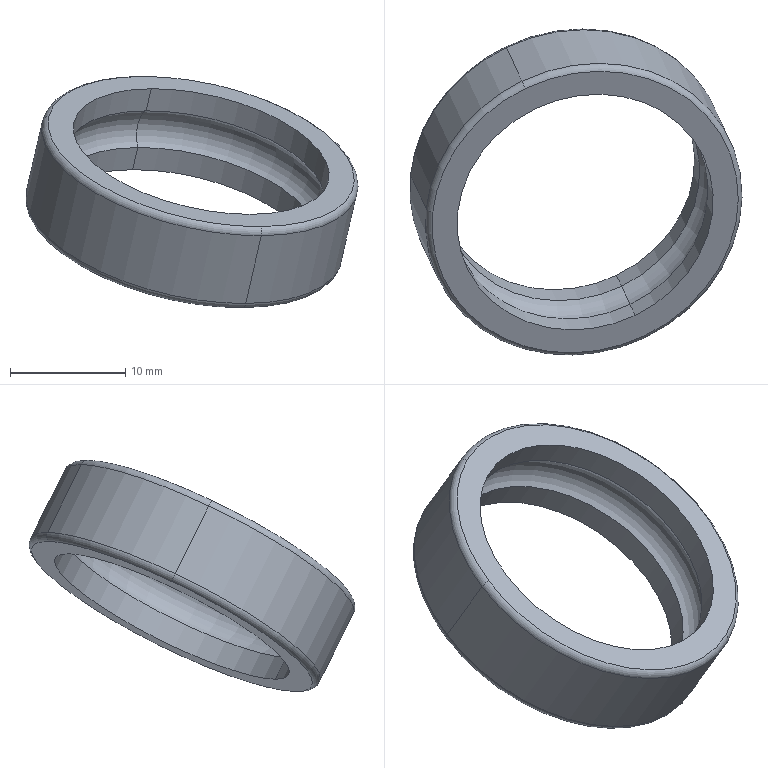Part | SolidWorks | features BaseBody 1 | 1 solid | 20 faces | box 28.804 x 28.259 x 20.047 mm | volume 1513 mm3 | cylinder 9 | torus 9 | plane 2 | commonest cylinder face diameters 22.668 x6 28 x3
STEP:
#1=CARTESIAN_POINT('',(1918.977,-164.664,836.807));
#2=VERTEX_POINT('',#1);
#3=CARTESIAN_POINT('',(1934.349,-173.615,828.827));
#4=VERTEX_POINT('',#3);
#5=CARTESIAN_POINT('',(1930.024,-164.664,834.27));
#6=DIRECTION('',(0.2015,-0.436,0.8771));
#7=DIRECTION('',(-0.3816,0.7898,0.4803));
#8=AXIS2_PLACEMENT_3D('',#5,#6,#7);
#9=CIRCLE('',#8,11.334);
#10=EDGE_CURVE('',#2,#4,#9,.T.);
#11=ORIENTED_EDGE('',*,*,#10,.F.);
#12=CARTESIAN_POINT('',(1919.418,-165.618,838.726));
#13=VERTEX_POINT('',#12);
#14=CARTESIAN_POINT('',(1918.965,-164.637,836.755));
#15=DIRECTION('',(0.2015,-0.436,0.8771));
#16=VECTOR('',#15,1000.);
#17=LINE('',#14,#16);
#18=EDGE_CURVE('',#2,#13,#17,.T.);
#19=ORIENTED_EDGE('',*,*,#18,.T.);
#20=CARTESIAN_POINT('',(1934.79,-174.569,830.746));
#21=VERTEX_POINT('',#20);
#22=CARTESIAN_POINT('',(1930.465,-165.618,836.189));
#23=DIRECTION('',(-0.2015,0.436,-0.8771));
#24=DIRECTION('',(0.3816,-0.7898,-0.4803));
#25=AXIS2_PLACEMENT_3D('',#22,#23,#24);
#26=CIRCLE('',#25,11.334);
#27=EDGE_CURVE('',#21,#13,#26,.T.);
#28=ORIENTED_EDGE('',*,*,#27,.F.);
#29=CARTESIAN_POINT('',(1934.349,-173.615,828.827));
#30=DIRECTION('',(-0.2015,0.436,-0.8771));
#31=VECTOR('',#30,1000.);
#32=LINE('',#29,#31);
#33=EDGE_CURVE('',#21,#4,#32,.T.);
#34=ORIENTED_EDGE('',*,*,#33,.T.);
#35=EDGE_LOOP('',(#11,#19,#28,#34));
#36=FACE_OUTER_BOUND('',#35,.T.);
#37=CARTESIAN_POINT('',(1930.012,-164.637,834.217));
#38=DIRECTION('',(0.2015,-0.436,0.8771));
#39=DIRECTION('',(-0.9746,0.,0.2239));
#40=AXIS2_PLACEMENT_3D('',#37,#38,#39);
#41=CYLINDRICAL_SURFACE('',#40,11.334);
#42=ADVANCED_FACE('',(#36),#41,.F.);
#43=CARTESIAN_POINT('',(1916.818,-164.664,837.303));
#44=VERTEX_POINT('',#43);
#45=CARTESIAN_POINT('',(1924.853,-153.962,840.777));
#46=VERTEX_POINT('',#45);
#47=CARTESIAN_POINT('',(1930.024,-164.664,834.27));
#48=DIRECTION('',(-0.2015,0.436,-0.8771));
#49=DIRECTION('',(0.3816,-0.7898,-0.4803));
#50=AXIS2_PLACEMENT_3D('',#47,#48,#49);
#51=CIRCLE('',#50,13.55);
#52=EDGE_CURVE('',#44,#46,#51,.T.);
#53=ORIENTED_EDGE('',*,*,#52,.F.);
#54=CARTESIAN_POINT('',(1916.51,-164.947,837.974));
#55=VERTEX_POINT('',#54);
#56=CARTESIAN_POINT('',(1917.187,-164.947,837.819));
#57=DIRECTION('',(0.09761,0.8999,0.425));
#58=DIRECTION('',(0.,-0.427,0.9043));
#59=AXIS2_PLACEMENT_3D('',#56,#57,#58);
#60=CIRCLE('',#59,0.6944);
#61=EDGE_CURVE('',#44,#55,#60,.T.);
#62=ORIENTED_EDGE('',*,*,#61,.T.);
#63=CARTESIAN_POINT('',(1924.812,-153.89,841.564));
#64=VERTEX_POINT('',#63);
#65=CARTESIAN_POINT('',(1930.155,-164.947,834.84));
#66=DIRECTION('',(-0.2015,0.436,-0.8771));
#67=DIRECTION('',(0.3816,-0.7898,-0.4803));
#68=AXIS2_PLACEMENT_3D('',#65,#66,#67);
#69=CIRCLE('',#68,14.);
#70=EDGE_CURVE('',#55,#64,#69,.T.);
#71=ORIENTED_EDGE('',*,*,#70,.T.);
#72=CARTESIAN_POINT('',(1925.077,-154.439,841.23));
#73=DIRECTION('',(0.9021,0.4315,0.007269));
#74=DIRECTION('',(-0.3816,0.7898,0.4803));
#75=AXIS2_PLACEMENT_3D('',#72,#73,#74);
#76=CIRCLE('',#75,0.6944);
#77=EDGE_CURVE('',#46,#64,#76,.T.);
#78=ORIENTED_EDGE('',*,*,#77,.F.);
#79=EDGE_LOOP('',(#53,#62,#71,#78));
#80=FACE_OUTER_BOUND('',#79,.T.);
#81=CARTESIAN_POINT('',(1930.155,-164.947,834.84));
#82=DIRECTION('',(0.2015,-0.436,0.8771));
#83=DIRECTION('',(-0.9746,0.,0.2239));
#84=AXIS2_PLACEMENT_3D('',#81,#82,#83);
#85=TOROIDAL_SURFACE('',#84,13.306,0.6944);
#86=ADVANCED_FACE('',(#80),#85,.T.);
#87=ORIENTED_EDGE('',*,*,#70,.F.);
#88=CARTESIAN_POINT('',(1917.86,-167.868,843.851));
#89=VERTEX_POINT('',#88);
#90=CARTESIAN_POINT('',(1916.483,-164.889,837.857));
#91=DIRECTION('',(0.2015,-0.436,0.8771));
#92=VECTOR('',#91,1000.);
#93=LINE('',#90,#92);
#94=EDGE_CURVE('',#55,#89,#93,.T.);
#95=ORIENTED_EDGE('',*,*,#94,.T.);
#96=CARTESIAN_POINT('',(1926.162,-156.812,847.44));
#97=VERTEX_POINT('',#96);
#98=CARTESIAN_POINT('',(1931.505,-167.868,840.717));
#99=DIRECTION('',(0.2015,-0.436,0.8771));
#100=DIRECTION('',(-0.3816,0.7898,0.4803));
#101=AXIS2_PLACEMENT_3D('',#98,#99,#100);
#102=CIRCLE('',#101,14.);
#103=EDGE_CURVE('',#97,#89,#102,.T.);
#104=ORIENTED_EDGE('',*,*,#103,.F.);
#105=CARTESIAN_POINT('',(1926.162,-156.812,847.44));
#106=DIRECTION('',(0.2015,-0.436,0.8771));
#107=VECTOR('',#106,1000.);
#108=LINE('',#105,#107);
#109=EDGE_CURVE('',#64,#97,#108,.T.);
#110=ORIENTED_EDGE('',*,*,#109,.F.);
#111=EDGE_LOOP('',(#87,#95,#104,#110));
#112=FACE_OUTER_BOUND('',#111,.T.);
#113=CARTESIAN_POINT('',(1930.128,-164.889,834.722));
#114=DIRECTION('',(0.2015,-0.436,0.8771));
#115=DIRECTION('',(-0.9746,0.,0.2239));
#116=AXIS2_PLACEMENT_3D('',#113,#114,#115);
#117=CYLINDRICAL_SURFACE('',#116,14.);
#118=ADVANCED_FACE('',(#112),#117,.T.);
#119=ORIENTED_EDGE('',*,*,#103,.T.);
#120=CARTESIAN_POINT('',(1918.429,-168.152,844.32));
#121=VERTEX_POINT('',#120);
#122=CARTESIAN_POINT('',(1918.537,-167.868,843.695));
#123=DIRECTION('',(0.09761,0.8999,0.425));
#124=DIRECTION('',(0.,-0.427,0.9043));
#125=AXIS2_PLACEMENT_3D('',#122,#123,#124);
#126=CIRCLE('',#125,0.6944);
#127=EDGE_CURVE('',#89,#121,#126,.T.);
#128=ORIENTED_EDGE('',*,*,#127,.T.);
#129=CARTESIAN_POINT('',(1926.465,-157.45,847.794));
#130=VERTEX_POINT('',#129);
#131=CARTESIAN_POINT('',(1931.636,-168.152,841.287));
#132=DIRECTION('',(0.2015,-0.436,0.8771));
#133=DIRECTION('',(-0.3816,0.7898,0.4803));
#134=AXIS2_PLACEMENT_3D('',#131,#132,#133);
#135=CIRCLE('',#134,13.55);
#136=EDGE_CURVE('',#130,#121,#135,.T.);
#137=ORIENTED_EDGE('',*,*,#136,.F.);
#138=CARTESIAN_POINT('',(1926.427,-157.36,847.107));
#139=DIRECTION('',(0.9021,0.4315,0.007269));
#140=DIRECTION('',(0.05425,-0.1301,0.99));
#141=AXIS2_PLACEMENT_3D('',#138,#139,#140);
#142=CIRCLE('',#141,0.6944);
#143=EDGE_CURVE('',#97,#130,#142,.T.);
#144=ORIENTED_EDGE('',*,*,#143,.F.);
#145=EDGE_LOOP('',(#119,#128,#137,#144));
#146=FACE_OUTER_BOUND('',#145,.T.);
#147=CARTESIAN_POINT('',(1931.505,-167.868,840.717));
#148=DIRECTION('',(0.2015,-0.436,0.8771));
#149=DIRECTION('',(-0.9746,0.,0.2239));
#150=AXIS2_PLACEMENT_3D('',#147,#148,#149);
#151=TOROIDAL_SURFACE('',#150,13.306,0.6944);
#152=ADVANCED_FACE('',(#146),#151,.T.);
#153=CARTESIAN_POINT('',(1920.148,-167.198,841.905));
#154=VERTEX_POINT('',#153);
#155=CARTESIAN_POINT('',(1935.52,-176.149,833.924));
#156=VERTEX_POINT('',#155);
#157=CARTESIAN_POINT('',(1931.195,-167.198,839.367));
#158=DIRECTION('',(0.2015,-0.436,0.8771));
#159=DIRECTION('',(-0.3816,0.7898,0.4803));
#160=AXIS2_PLACEMENT_3D('',#157,#158,#159);
#161=CIRCLE('',#160,11.334);
#162=EDGE_CURVE('',#154,#156,#161,.T.);
#163=ORIENTED_EDGE('',*,*,#162,.F.);
#164=CARTESIAN_POINT('',(1920.589,-168.152,843.824));
#165=VERTEX_POINT('',#164);
#166=CARTESIAN_POINT('',(1920.136,-167.171,841.852));
#167=DIRECTION('',(0.2015,-0.436,0.8771));
#168=VECTOR('',#167,1000.);
#169=LINE('',#166,#168);
#170=EDGE_CURVE('',#154,#165,#169,.T.);
#171=ORIENTED_EDGE('',*,*,#170,.T.);
#172=CARTESIAN_POINT('',(1935.961,-177.103,835.843));
#173=VERTEX_POINT('',#172);
#174=CARTESIAN_POINT('',(1931.636,-168.152,841.287));
#175=DIRECTION('',(-0.2015,0.436,-0.8771));
#176=DIRECTION('',(0.3816,-0.7898,-0.4803));
#177=AXIS2_PLACEMENT_3D('',#174,#175,#176);
#178=CIRCLE('',#177,11.334);
#179=EDGE_CURVE('',#173,#165,#178,.T.);
#180=ORIENTED_EDGE('',*,*,#179,.F.);
#181=CARTESIAN_POINT('',(1935.52,-176.149,833.924));
#182=DIRECTION('',(0.2015,-0.436,0.8771));
#183=VECTOR('',#182,1000.);
#184=LINE('',#181,#183);
#185=EDGE_CURVE('',#156,#173,#184,.T.);
#186=ORIENTED_EDGE('',*,*,#185,.F.);
#187=EDGE_LOOP('',(#163,#171,#180,#186));
#188=FACE_OUTER_BOUND('',#187,.T.);
#189=CARTESIAN_POINT('',(1931.183,-167.171,839.315));
#190=DIRECTION('',(0.2015,-0.436,0.8771));
#191=DIRECTION('',(-0.9746,0.,0.2239));
#192=AXIS2_PLACEMENT_3D('',#189,#190,#191);
#193=CYLINDRICAL_SURFACE('',#192,11.334);
#194=ADVANCED_FACE('',(#188),#193,.F.);
#195=ORIENTED_EDGE('',*,*,#27,.T.);
#196=CARTESIAN_POINT('',(1921.083,-166.408,840.017));
#197=DIRECTION('',(0.09761,0.8999,0.425));
#198=DIRECTION('',(0.,-0.427,0.9043));
#199=AXIS2_PLACEMENT_3D('',#196,#197,#198);
#200=CIRCLE('',#199,2.25);
#201=EDGE_CURVE('',#13,#154,#200,.T.);
#202=ORIENTED_EDGE('',*,*,#201,.T.);
#203=ORIENTED_EDGE('',*,*,#162,.T.);
#204=CARTESIAN_POINT('',(1934.646,-174.305,832.976));
#205=DIRECTION('',(0.9021,0.4315,0.007269));
#206=DIRECTION('',(0.3816,-0.7898,-0.4803));
#207=AXIS2_PLACEMENT_3D('',#204,#205,#206);
#208=CIRCLE('',#207,2.25);
#209=EDGE_CURVE('',#156,#21,#208,.T.);
#210=ORIENTED_EDGE('',*,*,#209,.T.);
#211=EDGE_LOOP('',(#195,#202,#203,#210));
#212=FACE_OUTER_BOUND('',#211,.T.);
#213=CARTESIAN_POINT('',(1930.83,-166.408,837.778));
#214=DIRECTION('',(0.2015,-0.436,0.8771));
#215=DIRECTION('',(-0.9746,0.,0.2239));
#216=AXIS2_PLACEMENT_3D('',#213,#214,#215);
#217=TOROIDAL_SURFACE('',#216,10.,2.25);
#218=ADVANCED_FACE('',(#212),#217,.F.);
#219=CARTESIAN_POINT('',(1926.14,-156.666,841.632));
#220=VERTEX_POINT('',#219);
#221=CARTESIAN_POINT('',(1926.87,-158.246,844.811));
#222=VERTEX_POINT('',#221);
#223=CARTESIAN_POINT('',(1927.014,-158.51,842.581));
#224=DIRECTION('',(0.9021,0.4315,0.007269));
#225=DIRECTION('',(-0.3816,0.7898,0.4803));
#226=AXIS2_PLACEMENT_3D('',#223,#224,#225);
#227=CIRCLE('',#226,2.25);
#228=EDGE_CURVE('',#220,#222,#227,.T.);
#229=ORIENTED_EDGE('',*,*,#228,.F.);
#230=CARTESIAN_POINT('',(1930.465,-165.618,836.189));
#231=DIRECTION('',(-0.2015,0.436,-0.8771));
#232=DIRECTION('',(-0.3816,0.7898,0.4803));
#233=AXIS2_PLACEMENT_3D('',#230,#231,#232);
#234=CIRCLE('',#233,11.334);
#235=EDGE_CURVE('',#220,#21,#234,.T.);
#236=ORIENTED_EDGE('',*,*,#235,.T.);
#237=ORIENTED_EDGE('',*,*,#209,.F.);
#238=CARTESIAN_POINT('',(1931.195,-167.198,839.367));
#239=DIRECTION('',(0.2015,-0.436,0.8771));
#240=DIRECTION('',(0.3816,-0.7898,-0.4803));
#241=AXIS2_PLACEMENT_3D('',#238,#239,#240);
#242=CIRCLE('',#241,11.334);
#243=EDGE_CURVE('',#156,#222,#242,.T.);
#244=ORIENTED_EDGE('',*,*,#243,.T.);
#245=EDGE_LOOP('',(#229,#236,#237,#244));
#246=FACE_OUTER_BOUND('',#245,.T.);
#247=CARTESIAN_POINT('',(1930.83,-166.408,837.778));
#248=DIRECTION('',(0.2015,-0.436,0.8771));
#249=DIRECTION('',(-0.9746,0.,0.2239));
#250=AXIS2_PLACEMENT_3D('',#247,#248,#249);
#251=TOROIDAL_SURFACE('',#250,10.,2.25);
#252=ADVANCED_FACE('',(#246),#251,.F.);
#253=ORIENTED_EDGE('',*,*,#201,.F.);
#254=CARTESIAN_POINT('',(1930.465,-165.618,836.189));
#255=DIRECTION('',(-0.2015,0.436,-0.8771));
#256=DIRECTION('',(0.3816,-0.7898,-0.4803));
#257=AXIS2_PLACEMENT_3D('',#254,#255,#256);
#258=CIRCLE('',#257,11.334);
#259=EDGE_CURVE('',#13,#220,#258,.T.);
#260=ORIENTED_EDGE('',*,*,#259,.T.);
#261=ORIENTED_EDGE('',*,*,#228,.T.);
#262=CARTESIAN_POINT('',(1931.195,-167.198,839.367));
#263=DIRECTION('',(0.2015,-0.436,0.8771));
#264=DIRECTION('',(-0.3816,0.7898,0.4803));
#265=AXIS2_PLACEMENT_3D('',#262,#263,#264);
#266=CIRCLE('',#265,11.334);
#267=EDGE_CURVE('',#222,#154,#266,.T.);
#268=ORIENTED_EDGE('',*,*,#267,.T.);
#269=EDGE_LOOP('',(#253,#260,#261,#268));
#270=FACE_OUTER_BOUND('',#269,.T.);
#271=CARTESIAN_POINT('',(1930.83,-166.408,837.778));
#272=DIRECTION('',(0.2015,-0.436,0.8771));
#273=DIRECTION('',(-0.9746,0.,0.2239));
#274=AXIS2_PLACEMENT_3D('',#271,#272,#273);
#275=TOROIDAL_SURFACE('',#274,10.,2.25);
#276=ADVANCED_FACE('',(#270),#275,.F.);
#277=ORIENTED_EDGE('',*,*,#170,.F.);
#278=ORIENTED_EDGE('',*,*,#267,.F.);
#279=CARTESIAN_POINT('',(1927.31,-159.2,846.73));
#280=VERTEX_POINT('',#279);
#281=CARTESIAN_POINT('',(1926.87,-158.246,844.811));
#282=DIRECTION('',(-0.2015,0.436,-0.8771));
#283=VECTOR('',#282,1000.);
#284=LINE('',#281,#283);
#285=EDGE_CURVE('',#280,#222,#284,.T.);
#286=ORIENTED_EDGE('',*,*,#285,.F.);
#287=CARTESIAN_POINT('',(1931.636,-168.152,841.287));
#288=DIRECTION('',(-0.2015,0.436,-0.8771));
#289=DIRECTION('',(0.3816,-0.7898,-0.4803));
#290=AXIS2_PLACEMENT_3D('',#287,#288,#289);
#291=CIRCLE('',#290,11.334);
#292=EDGE_CURVE('',#165,#280,#291,.T.);
#293=ORIENTED_EDGE('',*,*,#292,.F.);
#294=EDGE_LOOP('',(#277,#278,#286,#293));
#295=FACE_OUTER_BOUND('',#294,.T.);
#296=CARTESIAN_POINT('',(1931.183,-167.171,839.315));
#297=DIRECTION('',(0.2015,-0.436,0.8771));
#298=DIRECTION('',(-0.9746,0.,0.2239));
#299=AXIS2_PLACEMENT_3D('',#296,#297,#298);
#300=CYLINDRICAL_SURFACE('',#299,11.334);
#301=ADVANCED_FACE('',(#295),#300,.F.);
#302=ORIENTED_EDGE('',*,*,#243,.F.);
#303=ORIENTED_EDGE('',*,*,#185,.T.);
#304=CARTESIAN_POINT('',(1931.636,-168.152,841.287));
#305=DIRECTION('',(-0.2015,0.436,-0.8771));
#306=DIRECTION('',(-0.3816,0.7898,0.4803));
#307=AXIS2_PLACEMENT_3D('',#304,#305,#306);
#308=CIRCLE('',#307,11.334);
#309=EDGE_CURVE('',#280,#173,#308,.T.);
#310=ORIENTED_EDGE('',*,*,#309,.F.);
#311=ORIENTED_EDGE('',*,*,#285,.T.);
#312=EDGE_LOOP('',(#302,#303,#310,#311));
#313=FACE_OUTER_BOUND('',#312,.T.);
#314=CARTESIAN_POINT('',(1931.183,-167.171,839.315));
#315=DIRECTION('',(0.2015,-0.436,0.8771));
#316=DIRECTION('',(-0.9746,0.,0.2239));
#317=AXIS2_PLACEMENT_3D('',#314,#315,#316);
#318=CYLINDRICAL_SURFACE('',#317,11.334);
#319=ADVANCED_FACE('',(#313),#318,.F.);
#320=CARTESIAN_POINT('',(1936.806,-178.853,834.779));
#321=VERTEX_POINT('',#320);
#322=CARTESIAN_POINT('',(1931.636,-168.152,841.287));
#323=DIRECTION('',(0.2015,-0.436,0.8771));
#324=DIRECTION('',(0.3816,-0.7898,-0.4803));
#325=AXIS2_PLACEMENT_3D('',#322,#323,#324);
#326=CIRCLE('',#325,13.55);
#327=EDGE_CURVE('',#321,#130,#326,.T.);
#328=ORIENTED_EDGE('',*,*,#327,.T.);
#329=ORIENTED_EDGE('',*,*,#136,.T.);
#330=CARTESIAN_POINT('',(1931.636,-168.152,841.287));
#331=DIRECTION('',(0.2015,-0.436,0.8771));
#332=DIRECTION('',(-0.3816,0.7898,0.4803));
#333=AXIS2_PLACEMENT_3D('',#330,#331,#332);
#334=CIRCLE('',#333,13.55);
#335=EDGE_CURVE('',#121,#321,#334,.T.);
#336=ORIENTED_EDGE('',*,*,#335,.T.);
#337=EDGE_LOOP('',(#328,#329,#336));
#338=FACE_OUTER_BOUND('',#337,.T.);
#339=ORIENTED_EDGE('',*,*,#309,.T.);
#340=ORIENTED_EDGE('',*,*,#179,.T.);
#341=ORIENTED_EDGE('',*,*,#292,.T.);
#342=EDGE_LOOP('',(#339,#340,#341));
#343=FACE_BOUND('',#342,.T.);
#344=CARTESIAN_POINT('',(1919.275,-155.47,850.43));
#345=DIRECTION('',(0.2015,-0.436,0.8771));
#346=DIRECTION('',(-0.09761,-0.8999,-0.425));
#347=AXIS2_PLACEMENT_3D('',#344,#345,#346);
#348=PLANE('',#347);
#349=ADVANCED_FACE('',(#338,#343),#348,.T.);
#350=ORIENTED_EDGE('',*,*,#143,.T.);
#351=ORIENTED_EDGE('',*,*,#327,.F.);
#352=CARTESIAN_POINT('',(1936.847,-178.925,833.993));
#353=VERTEX_POINT('',#352);
#354=CARTESIAN_POINT('',(1936.582,-178.377,834.326));
#355=DIRECTION('',(0.9021,0.4315,0.007269));
#356=DIRECTION('',(0.3229,-0.6861,0.6519));
#357=AXIS2_PLACEMENT_3D('',#354,#355,#356);
#358=CIRCLE('',#357,0.6944);
#359=EDGE_CURVE('',#321,#353,#358,.T.);
#360=ORIENTED_EDGE('',*,*,#359,.T.);
#361=CARTESIAN_POINT('',(1931.505,-167.868,840.717));
#362=DIRECTION('',(0.2015,-0.436,0.8771));
#363=DIRECTION('',(0.3816,-0.7898,-0.4803));
#364=AXIS2_PLACEMENT_3D('',#361,#362,#363);
#365=CIRCLE('',#364,14.);
#366=EDGE_CURVE('',#353,#97,#365,.T.);
#367=ORIENTED_EDGE('',*,*,#366,.T.);
#368=EDGE_LOOP('',(#350,#351,#360,#367));
#369=FACE_OUTER_BOUND('',#368,.T.);
#370=CARTESIAN_POINT('',(1931.505,-167.868,840.717));
#371=DIRECTION('',(0.2015,-0.436,0.8771));
#372=DIRECTION('',(-0.9746,0.,0.2239));
#373=AXIS2_PLACEMENT_3D('',#370,#371,#372);
#374=TOROIDAL_SURFACE('',#373,13.306,0.6944);
#375=ADVANCED_FACE('',(#369),#374,.T.);
#376=ORIENTED_EDGE('',*,*,#127,.F.);
#377=CARTESIAN_POINT('',(1931.505,-167.868,840.717));
#378=DIRECTION('',(0.2015,-0.436,0.8771));
#379=DIRECTION('',(-0.3816,0.7898,0.4803));
#380=AXIS2_PLACEMENT_3D('',#377,#378,#379);
#381=CIRCLE('',#380,14.);
#382=EDGE_CURVE('',#89,#353,#381,.T.);
#383=ORIENTED_EDGE('',*,*,#382,.T.);
#384=ORIENTED_EDGE('',*,*,#359,.F.);
#385=ORIENTED_EDGE('',*,*,#335,.F.);
#386=EDGE_LOOP('',(#376,#383,#384,#385));
#387=FACE_OUTER_BOUND('',#386,.T.);
#388=CARTESIAN_POINT('',(1931.505,-167.868,840.717));
#389=DIRECTION('',(0.2015,-0.436,0.8771));
#390=DIRECTION('',(-0.9746,0.,0.2239));
#391=AXIS2_PLACEMENT_3D('',#388,#389,#390);
#392=TOROIDAL_SURFACE('',#391,13.306,0.6944);
#393=ADVANCED_FACE('',(#387),#392,.T.);
#394=ORIENTED_EDGE('',*,*,#94,.F.);
#395=CARTESIAN_POINT('',(1935.497,-176.004,828.116));
#396=VERTEX_POINT('',#395);
#397=CARTESIAN_POINT('',(1930.155,-164.947,834.84));
#398=DIRECTION('',(-0.2015,0.436,-0.8771));
#399=DIRECTION('',(0.3816,-0.7898,-0.4803));
#400=AXIS2_PLACEMENT_3D('',#397,#398,#399);
#401=CIRCLE('',#400,14.);
#402=EDGE_CURVE('',#396,#55,#401,.T.);
#403=ORIENTED_EDGE('',*,*,#402,.F.);
#404=CARTESIAN_POINT('',(1936.847,-178.925,833.993));
#405=DIRECTION('',(-0.2015,0.436,-0.8771));
#406=VECTOR('',#405,1000.);
#407=LINE('',#404,#406);
#408=EDGE_CURVE('',#353,#396,#407,.T.);
#409=ORIENTED_EDGE('',*,*,#408,.F.);
#410=ORIENTED_EDGE('',*,*,#382,.F.);
#411=EDGE_LOOP('',(#394,#403,#409,#410));
#412=FACE_OUTER_BOUND('',#411,.T.);
#413=CARTESIAN_POINT('',(1930.128,-164.889,834.722));
#414=DIRECTION('',(0.2015,-0.436,0.8771));
#415=DIRECTION('',(-0.9746,0.,0.2239));
#416=AXIS2_PLACEMENT_3D('',#413,#414,#415);
#417=CYLINDRICAL_SURFACE('',#416,14.);
#418=ADVANCED_FACE('',(#412),#417,.T.);
#419=ORIENTED_EDGE('',*,*,#366,.F.);
#420=ORIENTED_EDGE('',*,*,#408,.T.);
#421=CARTESIAN_POINT('',(1930.155,-164.947,834.84));
#422=DIRECTION('',(-0.2015,0.436,-0.8771));
#423=DIRECTION('',(-0.3816,0.7898,0.4803));
#424=AXIS2_PLACEMENT_3D('',#421,#422,#423);
#425=CIRCLE('',#424,14.);
#426=EDGE_CURVE('',#64,#396,#425,.T.);
#427=ORIENTED_EDGE('',*,*,#426,.F.);
#428=ORIENTED_EDGE('',*,*,#109,.T.);
#429=EDGE_LOOP('',(#419,#420,#427,#428));
#430=FACE_OUTER_BOUND('',#429,.T.);
#431=CARTESIAN_POINT('',(1930.128,-164.889,834.722));
#432=DIRECTION('',(0.2015,-0.436,0.8771));
#433=DIRECTION('',(-0.9746,0.,0.2239));
#434=AXIS2_PLACEMENT_3D('',#431,#432,#433);
#435=CYLINDRICAL_SURFACE('',#434,14.);
#436=ADVANCED_FACE('',(#430),#435,.T.);
#437=ORIENTED_EDGE('',*,*,#426,.T.);
#438=CARTESIAN_POINT('',(1935.194,-175.365,827.762));
#439=VERTEX_POINT('',#438);
#440=CARTESIAN_POINT('',(1935.232,-175.455,828.45));
#441=DIRECTION('',(0.9021,0.4315,0.007269));
#442=DIRECTION('',(0.3816,-0.7898,-0.4803));
#443=AXIS2_PLACEMENT_3D('',#440,#441,#442);
#444=CIRCLE('',#443,0.6944);
#445=EDGE_CURVE('',#396,#439,#444,.T.);
#446=ORIENTED_EDGE('',*,*,#445,.T.);
#447=CARTESIAN_POINT('',(1930.024,-164.664,834.27));
#448=DIRECTION('',(-0.2015,0.436,-0.8771));
#449=DIRECTION('',(-0.3816,0.7898,0.4803));
#450=AXIS2_PLACEMENT_3D('',#447,#448,#449);
#451=CIRCLE('',#450,13.55);
#452=EDGE_CURVE('',#46,#439,#451,.T.);
#453=ORIENTED_EDGE('',*,*,#452,.F.);
#454=ORIENTED_EDGE('',*,*,#77,.T.);
#455=EDGE_LOOP('',(#437,#446,#453,#454));
#456=FACE_OUTER_BOUND('',#455,.T.);
#457=CARTESIAN_POINT('',(1930.155,-164.947,834.84));
#458=DIRECTION('',(0.2015,-0.436,0.8771));
#459=DIRECTION('',(-0.9746,0.,0.2239));
#460=AXIS2_PLACEMENT_3D('',#457,#458,#459);
#461=TOROIDAL_SURFACE('',#460,13.306,0.6944);
#462=ADVANCED_FACE('',(#456),#461,.T.);
#463=ORIENTED_EDGE('',*,*,#61,.F.);
#464=CARTESIAN_POINT('',(1930.024,-164.664,834.27));
#465=DIRECTION('',(-0.2015,0.436,-0.8771));
#466=DIRECTION('',(0.3816,-0.7898,-0.4803));
#467=AXIS2_PLACEMENT_3D('',#464,#465,#466);
#468=CIRCLE('',#467,13.55);
#469=EDGE_CURVE('',#439,#44,#468,.T.);
#470=ORIENTED_EDGE('',*,*,#469,.F.);
#471=ORIENTED_EDGE('',*,*,#445,.F.);
#472=ORIENTED_EDGE('',*,*,#402,.T.);
#473=EDGE_LOOP('',(#463,#470,#471,#472));
#474=FACE_OUTER_BOUND('',#473,.T.);
#475=CARTESIAN_POINT('',(1930.155,-164.947,834.84));
#476=DIRECTION('',(0.2015,-0.436,0.8771));
#477=DIRECTION('',(-0.9746,0.,0.2239));
#478=AXIS2_PLACEMENT_3D('',#475,#476,#477);
#479=TOROIDAL_SURFACE('',#478,13.306,0.6944);
#480=ADVANCED_FACE('',(#474),#479,.T.);
#481=ORIENTED_EDGE('',*,*,#452,.T.);
#482=ORIENTED_EDGE('',*,*,#469,.T.);
#483=ORIENTED_EDGE('',*,*,#52,.T.);
#484=EDGE_LOOP('',(#481,#482,#483));
#485=FACE_OUTER_BOUND('',#484,.T.);
#486=CARTESIAN_POINT('',(1925.699,-155.712,839.713));
#487=VERTEX_POINT('',#486);
#488=CARTESIAN_POINT('',(1930.024,-164.664,834.27));
#489=DIRECTION('',(0.2015,-0.436,0.8771));
#490=DIRECTION('',(0.3816,-0.7898,-0.4803));
#491=AXIS2_PLACEMENT_3D('',#488,#489,#490);
#492=CIRCLE('',#491,11.334);
#493=EDGE_CURVE('',#4,#487,#492,.T.);
#494=ORIENTED_EDGE('',*,*,#493,.T.);
#495=CARTESIAN_POINT('',(1930.024,-164.664,834.27));
#496=DIRECTION('',(0.2015,-0.436,0.8771));
#497=DIRECTION('',(-0.3816,0.7898,0.4803));
#498=AXIS2_PLACEMENT_3D('',#495,#496,#497);
#499=CIRCLE('',#498,11.334);
#500=EDGE_CURVE('',#487,#2,#499,.T.);
#501=ORIENTED_EDGE('',*,*,#500,.T.);
#502=ORIENTED_EDGE('',*,*,#10,.T.);
#503=EDGE_LOOP('',(#494,#501,#502));
#504=FACE_BOUND('',#503,.T.);
#505=CARTESIAN_POINT('',(1917.664,-151.98,843.414));
#506=DIRECTION('',(-0.2015,0.436,-0.8771));
#507=DIRECTION('',(0.9746,0.,-0.2239));
#508=AXIS2_PLACEMENT_3D('',#505,#506,#507);
#509=PLANE('',#508);
#510=ADVANCED_FACE('',(#485,#504),#509,.T.);
#511=CARTESIAN_POINT('',(1925.699,-155.712,839.713));
#512=DIRECTION('',(0.2015,-0.436,0.8771));
#513=VECTOR('',#512,1000.);
#514=LINE('',#511,#513);
#515=EDGE_CURVE('',#487,#220,#514,.T.);
#516=ORIENTED_EDGE('',*,*,#515,.F.);
#517=ORIENTED_EDGE('',*,*,#493,.F.);
#518=ORIENTED_EDGE('',*,*,#33,.F.);
#519=ORIENTED_EDGE('',*,*,#235,.F.);
#520=EDGE_LOOP('',(#516,#517,#518,#519));
#521=FACE_OUTER_BOUND('',#520,.T.);
#522=CARTESIAN_POINT('',(1930.012,-164.637,834.217));
#523=DIRECTION('',(0.2015,-0.436,0.8771));
#524=DIRECTION('',(-0.9746,0.,0.2239));
#525=AXIS2_PLACEMENT_3D('',#522,#523,#524);
#526=CYLINDRICAL_SURFACE('',#525,11.334);
#527=ADVANCED_FACE('',(#521),#526,.F.);
#528=ORIENTED_EDGE('',*,*,#18,.F.);
#529=ORIENTED_EDGE('',*,*,#500,.F.);
#530=ORIENTED_EDGE('',*,*,#515,.T.);
#531=ORIENTED_EDGE('',*,*,#259,.F.);
#532=EDGE_LOOP('',(#528,#529,#530,#531));
#533=FACE_OUTER_BOUND('',#532,.T.);
#534=CARTESIAN_POINT('',(1930.012,-164.637,834.217));
#535=DIRECTION('',(0.2015,-0.436,0.8771));
#536=DIRECTION('',(-0.9746,0.,0.2239));
#537=AXIS2_PLACEMENT_3D('',#534,#535,#536);
#538=CYLINDRICAL_SURFACE('',#537,11.334);
#539=ADVANCED_FACE('',(#533),#538,.F.);
#540=CLOSED_SHELL('',(#42,#86,#118,#152,#194,#218,#252,#276,#301,#319,#349,#375,#393,#418,#436,#462,#480,#510,#527,#539));
#541=MANIFOLD_SOLID_BREP('',#540);
#542=CARTESIAN_POINT('',(0.,0.,0.));
#543=DIRECTION('',(0.,0.,1.));
#544=DIRECTION('',(1.,0.,0.));
#545=AXIS2_PLACEMENT_3D('',#542,#543,#544);
#546=(LENGTH_UNIT()NAMED_UNIT(*)SI_UNIT(.MILLI.,.METRE.));
#547=UNCERTAINTY_MEASURE_WITH_UNIT(LENGTH_MEASURE(0.00001),#546,'','');
#548=(NAMED_UNIT(*)PLANE_ANGLE_UNIT()SI_UNIT($,.RADIAN.));
#549=(NAMED_UNIT(*)SI_UNIT($,.STERADIAN.)SOLID_ANGLE_UNIT());
#550=(GEOMETRIC_REPRESENTATION_CONTEXT(3)GLOBAL_UNCERTAINTY_ASSIGNED_CONTEXT((#547))GLOBAL_UNIT_ASSIGNED_CONTEXT((#546,#548,#549))REPRESENTATION_CONTEXT('',''));
#551=ADVANCED_BREP_SHAPE_REPRESENTATION('',(#541,#545),#550);